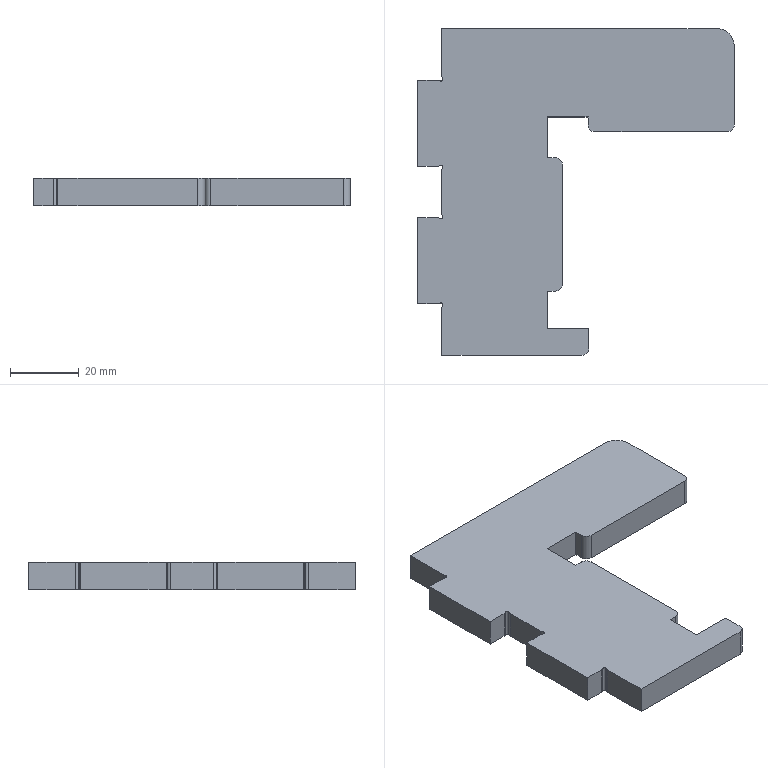Part | SolidWorks | features Fillet 2, FlatPattern 1, ICE 1, SMBaseFlange 1, SheetMetal 1 | 1 solid | 46 faces | box 92 x 95 x 8 mm | volume 40763 mm3 | plane 24 | cylinder 22 | commonest cylinder face diameters 4 x13 1 x8 10 x1
STEP:
#1=CARTESIAN_POINT('',(-1503.95,-54.15,0.));
#2=VERTEX_POINT('',#1);
#3=CARTESIAN_POINT('',(-1504.668,-53.7,0.));
#4=VERTEX_POINT('',#3);
#5=CARTESIAN_POINT('',(-1504.45,-54.15,0.));
#6=DIRECTION('',(0.,0.,1.));
#7=DIRECTION('',(1.,0.,0.));
#8=AXIS2_PLACEMENT_3D('',#5,#6,#7);
#9=CIRCLE('',#8,0.5);
#10=EDGE_CURVE('',#2,#4,#9,.T.);
#11=ORIENTED_EDGE('',*,*,#10,.F.);
#12=CARTESIAN_POINT('',(-1503.95,-54.15,8.));
#13=VERTEX_POINT('',#12);
#14=CARTESIAN_POINT('',(-1503.95,-54.15,0.));
#15=DIRECTION('',(0.,0.,1.));
#16=VECTOR('',#15,1000.);
#17=LINE('',#14,#16);
#18=EDGE_CURVE('',#2,#13,#17,.T.);
#19=ORIENTED_EDGE('',*,*,#18,.T.);
#20=CARTESIAN_POINT('',(-1504.668,-53.7,8.));
#21=VERTEX_POINT('',#20);
#22=CARTESIAN_POINT('',(-1504.45,-54.15,8.));
#23=DIRECTION('',(0.,0.,1.));
#24=DIRECTION('',(1.,0.,0.));
#25=AXIS2_PLACEMENT_3D('',#22,#23,#24);
#26=CIRCLE('',#25,0.5);
#27=EDGE_CURVE('',#13,#21,#26,.T.);
#28=ORIENTED_EDGE('',*,*,#27,.T.);
#29=CARTESIAN_POINT('',(-1504.668,-53.7,0.));
#30=DIRECTION('',(0.,0.,-1.));
#31=VECTOR('',#30,1000.);
#32=LINE('',#29,#31);
#33=EDGE_CURVE('',#21,#4,#32,.T.);
#34=ORIENTED_EDGE('',*,*,#33,.T.);
#35=EDGE_LOOP('',(#11,#19,#28,#34));
#36=FACE_OUTER_BOUND('',#35,.T.);
#37=CARTESIAN_POINT('',(-1504.45,-54.15,0.));
#38=DIRECTION('',(0.,0.,1.));
#39=DIRECTION('',(1.,0.,0.));
#40=AXIS2_PLACEMENT_3D('',#37,#38,#39);
#41=CYLINDRICAL_SURFACE('',#40,0.5);
#42=ADVANCED_FACE('',(#36),#41,.F.);
#43=CARTESIAN_POINT('',(-1503.95,11.35,0.));
#44=VERTEX_POINT('',#43);
#45=CARTESIAN_POINT('',(-1504.,11.568,0.));
#46=VERTEX_POINT('',#45);
#47=CARTESIAN_POINT('',(-1504.45,11.35,0.));
#48=DIRECTION('',(0.,0.,1.));
#49=DIRECTION('',(1.,0.,0.));
#50=AXIS2_PLACEMENT_3D('',#47,#48,#49);
#51=CIRCLE('',#50,0.5);
#52=EDGE_CURVE('',#44,#46,#51,.T.);
#53=ORIENTED_EDGE('',*,*,#52,.F.);
#54=CARTESIAN_POINT('',(-1503.95,11.35,8.));
#55=VERTEX_POINT('',#54);
#56=CARTESIAN_POINT('',(-1503.95,11.35,0.));
#57=DIRECTION('',(0.,0.,1.));
#58=VECTOR('',#57,1000.);
#59=LINE('',#56,#58);
#60=EDGE_CURVE('',#44,#55,#59,.T.);
#61=ORIENTED_EDGE('',*,*,#60,.T.);
#62=CARTESIAN_POINT('',(-1504.,11.568,8.));
#63=VERTEX_POINT('',#62);
#64=CARTESIAN_POINT('',(-1504.45,11.35,8.));
#65=DIRECTION('',(0.,0.,1.));
#66=DIRECTION('',(1.,0.,0.));
#67=AXIS2_PLACEMENT_3D('',#64,#65,#66);
#68=CIRCLE('',#67,0.5);
#69=EDGE_CURVE('',#55,#63,#68,.T.);
#70=ORIENTED_EDGE('',*,*,#69,.T.);
#71=CARTESIAN_POINT('',(-1504.,11.568,0.));
#72=DIRECTION('',(0.,0.,-1.));
#73=VECTOR('',#72,1000.);
#74=LINE('',#71,#73);
#75=EDGE_CURVE('',#63,#46,#74,.T.);
#76=ORIENTED_EDGE('',*,*,#75,.T.);
#77=EDGE_LOOP('',(#53,#61,#70,#76));
#78=FACE_OUTER_BOUND('',#77,.T.);
#79=CARTESIAN_POINT('',(-1504.45,11.35,0.));
#80=DIRECTION('',(0.,0.,1.));
#81=DIRECTION('',(1.,0.,0.));
#82=AXIS2_PLACEMENT_3D('',#79,#80,#81);
#83=CYLINDRICAL_SURFACE('',#82,0.5);
#84=ADVANCED_FACE('',(#78),#83,.F.);
#85=CARTESIAN_POINT('',(-1503.95,-14.15,0.));
#86=VERTEX_POINT('',#85);
#87=CARTESIAN_POINT('',(-1504.668,-13.7,0.));
#88=VERTEX_POINT('',#87);
#89=CARTESIAN_POINT('',(-1504.45,-14.15,0.));
#90=DIRECTION('',(0.,0.,1.));
#91=DIRECTION('',(1.,0.,0.));
#92=AXIS2_PLACEMENT_3D('',#89,#90,#91);
#93=CIRCLE('',#92,0.5);
#94=EDGE_CURVE('',#86,#88,#93,.T.);
#95=ORIENTED_EDGE('',*,*,#94,.F.);
#96=CARTESIAN_POINT('',(-1503.95,-14.15,8.));
#97=VERTEX_POINT('',#96);
#98=CARTESIAN_POINT('',(-1503.95,-14.15,0.));
#99=DIRECTION('',(0.,0.,1.));
#100=VECTOR('',#99,1000.);
#101=LINE('',#98,#100);
#102=EDGE_CURVE('',#86,#97,#101,.T.);
#103=ORIENTED_EDGE('',*,*,#102,.T.);
#104=CARTESIAN_POINT('',(-1504.668,-13.7,8.));
#105=VERTEX_POINT('',#104);
#106=CARTESIAN_POINT('',(-1504.45,-14.15,8.));
#107=DIRECTION('',(0.,0.,1.));
#108=DIRECTION('',(1.,0.,0.));
#109=AXIS2_PLACEMENT_3D('',#106,#107,#108);
#110=CIRCLE('',#109,0.5);
#111=EDGE_CURVE('',#97,#105,#110,.T.);
#112=ORIENTED_EDGE('',*,*,#111,.T.);
#113=CARTESIAN_POINT('',(-1504.668,-13.7,0.));
#114=DIRECTION('',(0.,0.,-1.));
#115=VECTOR('',#114,1000.);
#116=LINE('',#113,#115);
#117=EDGE_CURVE('',#105,#88,#116,.T.);
#118=ORIENTED_EDGE('',*,*,#117,.T.);
#119=EDGE_LOOP('',(#95,#103,#112,#118));
#120=FACE_OUTER_BOUND('',#119,.T.);
#121=CARTESIAN_POINT('',(-1504.45,-14.15,0.));
#122=DIRECTION('',(0.,0.,1.));
#123=DIRECTION('',(1.,0.,0.));
#124=AXIS2_PLACEMENT_3D('',#121,#122,#123);
#125=CYLINDRICAL_SURFACE('',#124,0.5);
#126=ADVANCED_FACE('',(#120),#125,.F.);
#127=CARTESIAN_POINT('',(-1503.95,-28.648,0.));
#128=VERTEX_POINT('',#127);
#129=CARTESIAN_POINT('',(-1504.,-28.43,0.));
#130=VERTEX_POINT('',#129);
#131=CARTESIAN_POINT('',(-1504.45,-28.648,0.));
#132=DIRECTION('',(0.,0.,1.));
#133=DIRECTION('',(1.,0.,0.));
#134=AXIS2_PLACEMENT_3D('',#131,#132,#133);
#135=CIRCLE('',#134,0.5);
#136=EDGE_CURVE('',#128,#130,#135,.T.);
#137=ORIENTED_EDGE('',*,*,#136,.F.);
#138=CARTESIAN_POINT('',(-1503.95,-28.648,8.));
#139=VERTEX_POINT('',#138);
#140=CARTESIAN_POINT('',(-1503.95,-28.648,0.));
#141=DIRECTION('',(0.,0.,1.));
#142=VECTOR('',#141,1000.);
#143=LINE('',#140,#142);
#144=EDGE_CURVE('',#128,#139,#143,.T.);
#145=ORIENTED_EDGE('',*,*,#144,.T.);
#146=CARTESIAN_POINT('',(-1504.,-28.43,8.));
#147=VERTEX_POINT('',#146);
#148=CARTESIAN_POINT('',(-1504.45,-28.648,8.));
#149=DIRECTION('',(0.,0.,1.));
#150=DIRECTION('',(1.,0.,0.));
#151=AXIS2_PLACEMENT_3D('',#148,#149,#150);
#152=CIRCLE('',#151,0.5);
#153=EDGE_CURVE('',#139,#147,#152,.T.);
#154=ORIENTED_EDGE('',*,*,#153,.T.);
#155=CARTESIAN_POINT('',(-1504.,-28.43,0.));
#156=DIRECTION('',(0.,0.,-1.));
#157=VECTOR('',#156,1000.);
#158=LINE('',#155,#157);
#159=EDGE_CURVE('',#147,#130,#158,.T.);
#160=ORIENTED_EDGE('',*,*,#159,.T.);
#161=EDGE_LOOP('',(#137,#145,#154,#160));
#162=FACE_OUTER_BOUND('',#161,.T.);
#163=CARTESIAN_POINT('',(-1504.45,-28.648,0.));
#164=DIRECTION('',(0.,0.,1.));
#165=DIRECTION('',(1.,0.,0.));
#166=AXIS2_PLACEMENT_3D('',#163,#164,#165);
#167=CYLINDRICAL_SURFACE('',#166,0.5);
#168=ADVANCED_FACE('',(#162),#167,.F.);
#169=CARTESIAN_POINT('',(-1504.2,26.1,0.));
#170=VERTEX_POINT('',#169);
#171=CARTESIAN_POINT('',(-1504.2,12.44,0.));
#172=VERTEX_POINT('',#171);
#173=CARTESIAN_POINT('',(-1504.2,26.1,0.));
#174=DIRECTION('',(0.,-1.,0.));
#175=VECTOR('',#174,1000.);
#176=LINE('',#173,#175);
#177=EDGE_CURVE('',#170,#172,#176,.T.);
#178=ORIENTED_EDGE('',*,*,#177,.T.);
#179=CARTESIAN_POINT('',(-1504.2,12.44,8.));
#180=VERTEX_POINT('',#179);
#181=CARTESIAN_POINT('',(-1504.2,12.44,8.));
#182=DIRECTION('',(0.,0.,1.));
#183=VECTOR('',#182,1000.);
#184=LINE('',#181,#183);
#185=EDGE_CURVE('',#172,#180,#184,.T.);
#186=ORIENTED_EDGE('',*,*,#185,.T.);
#187=CARTESIAN_POINT('',(-1504.2,26.1,8.));
#188=VERTEX_POINT('',#187);
#189=CARTESIAN_POINT('',(-1504.2,26.1,8.));
#190=DIRECTION('',(0.,-1.,0.));
#191=VECTOR('',#190,1000.);
#192=LINE('',#189,#191);
#193=EDGE_CURVE('',#188,#180,#192,.T.);
#194=ORIENTED_EDGE('',*,*,#193,.F.);
#195=CARTESIAN_POINT('',(-1504.2,26.1,8.));
#196=DIRECTION('',(0.,0.,-1.));
#197=VECTOR('',#196,1000.);
#198=LINE('',#195,#197);
#199=EDGE_CURVE('',#188,#170,#198,.T.);
#200=ORIENTED_EDGE('',*,*,#199,.T.);
#201=EDGE_LOOP('',(#178,#186,#194,#200));
#202=FACE_OUTER_BOUND('',#201,.T.);
#203=CARTESIAN_POINT('',(-1504.2,26.1,8.));
#204=DIRECTION('',(1.,0.,0.));
#205=DIRECTION('',(0.,0.,-1.));
#206=AXIS2_PLACEMENT_3D('',#203,#204,#205);
#207=PLANE('',#206);
#208=ADVANCED_FACE('',(#202),#207,.F.);
#209=CARTESIAN_POINT('',(-1505.54,11.1,8.));
#210=VERTEX_POINT('',#209);
#211=CARTESIAN_POINT('',(-1511.2,11.1,8.));
#212=VERTEX_POINT('',#211);
#213=CARTESIAN_POINT('',(-1511.2,11.1,8.));
#214=DIRECTION('',(-1.,0.,0.));
#215=VECTOR('',#214,1000.);
#216=LINE('',#213,#215);
#217=EDGE_CURVE('',#210,#212,#216,.T.);
#218=ORIENTED_EDGE('',*,*,#217,.F.);
#219=CARTESIAN_POINT('',(-1505.54,11.1,0.));
#220=VERTEX_POINT('',#219);
#221=CARTESIAN_POINT('',(-1505.54,11.1,0.));
#222=DIRECTION('',(0.,0.,-1.));
#223=VECTOR('',#222,1000.);
#224=LINE('',#221,#223);
#225=EDGE_CURVE('',#210,#220,#224,.T.);
#226=ORIENTED_EDGE('',*,*,#225,.T.);
#227=CARTESIAN_POINT('',(-1511.2,11.1,0.));
#228=VERTEX_POINT('',#227);
#229=CARTESIAN_POINT('',(-1511.2,11.1,0.));
#230=DIRECTION('',(-1.,0.,0.));
#231=VECTOR('',#230,1000.);
#232=LINE('',#229,#231);
#233=EDGE_CURVE('',#220,#228,#232,.T.);
#234=ORIENTED_EDGE('',*,*,#233,.T.);
#235=CARTESIAN_POINT('',(-1511.2,11.1,8.));
#236=DIRECTION('',(0.,0.,-1.));
#237=VECTOR('',#236,1000.);
#238=LINE('',#235,#237);
#239=EDGE_CURVE('',#212,#228,#238,.T.);
#240=ORIENTED_EDGE('',*,*,#239,.F.);
#241=EDGE_LOOP('',(#218,#226,#234,#240));
#242=FACE_OUTER_BOUND('',#241,.T.);
#243=CARTESIAN_POINT('',(-1511.2,11.1,8.));
#244=DIRECTION('',(0.,-1.,0.));
#245=DIRECTION('',(0.,0.,-1.));
#246=AXIS2_PLACEMENT_3D('',#243,#244,#245);
#247=PLANE('',#246);
#248=ADVANCED_FACE('',(#242),#247,.F.);
#249=CARTESIAN_POINT('',(-1511.2,-13.9,0.));
#250=VERTEX_POINT('',#249);
#251=CARTESIAN_POINT('',(-1505.54,-13.9,0.));
#252=VERTEX_POINT('',#251);
#253=CARTESIAN_POINT('',(-1504.2,-13.9,0.));
#254=DIRECTION('',(1.,0.,0.));
#255=VECTOR('',#254,1000.);
#256=LINE('',#253,#255);
#257=EDGE_CURVE('',#250,#252,#256,.T.);
#258=ORIENTED_EDGE('',*,*,#257,.T.);
#259=CARTESIAN_POINT('',(-1505.54,-13.9,8.));
#260=VERTEX_POINT('',#259);
#261=CARTESIAN_POINT('',(-1505.54,-13.9,8.));
#262=DIRECTION('',(0.,0.,1.));
#263=VECTOR('',#262,1000.);
#264=LINE('',#261,#263);
#265=EDGE_CURVE('',#252,#260,#264,.T.);
#266=ORIENTED_EDGE('',*,*,#265,.T.);
#267=CARTESIAN_POINT('',(-1511.2,-13.9,8.));
#268=VERTEX_POINT('',#267);
#269=CARTESIAN_POINT('',(-1504.2,-13.9,8.));
#270=DIRECTION('',(1.,0.,0.));
#271=VECTOR('',#270,1000.);
#272=LINE('',#269,#271);
#273=EDGE_CURVE('',#268,#260,#272,.T.);
#274=ORIENTED_EDGE('',*,*,#273,.F.);
#275=CARTESIAN_POINT('',(-1511.2,-13.9,8.));
#276=DIRECTION('',(0.,0.,-1.));
#277=VECTOR('',#276,1000.);
#278=LINE('',#275,#277);
#279=EDGE_CURVE('',#268,#250,#278,.T.);
#280=ORIENTED_EDGE('',*,*,#279,.T.);
#281=EDGE_LOOP('',(#258,#266,#274,#280));
#282=FACE_OUTER_BOUND('',#281,.T.);
#283=CARTESIAN_POINT('',(-1504.2,-13.9,8.));
#284=DIRECTION('',(0.,1.,0.));
#285=DIRECTION('',(0.,0.,1.));
#286=AXIS2_PLACEMENT_3D('',#283,#284,#285);
#287=PLANE('',#286);
#288=ADVANCED_FACE('',(#282),#287,.F.);
#289=CARTESIAN_POINT('',(-1504.2,-15.24,8.));
#290=VERTEX_POINT('',#289);
#291=CARTESIAN_POINT('',(-1504.2,-27.558,8.));
#292=VERTEX_POINT('',#291);
#293=CARTESIAN_POINT('',(-1504.2,-13.9,8.));
#294=DIRECTION('',(0.,-1.,0.));
#295=VECTOR('',#294,1000.);
#296=LINE('',#293,#295);
#297=EDGE_CURVE('',#290,#292,#296,.T.);
#298=ORIENTED_EDGE('',*,*,#297,.F.);
#299=CARTESIAN_POINT('',(-1504.2,-15.24,0.));
#300=VERTEX_POINT('',#299);
#301=CARTESIAN_POINT('',(-1504.2,-15.24,0.));
#302=DIRECTION('',(0.,0.,-1.));
#303=VECTOR('',#302,1000.);
#304=LINE('',#301,#303);
#305=EDGE_CURVE('',#290,#300,#304,.T.);
#306=ORIENTED_EDGE('',*,*,#305,.T.);
#307=CARTESIAN_POINT('',(-1504.2,-27.558,0.));
#308=VERTEX_POINT('',#307);
#309=CARTESIAN_POINT('',(-1504.2,-13.9,0.));
#310=DIRECTION('',(0.,-1.,0.));
#311=VECTOR('',#310,1000.);
#312=LINE('',#309,#311);
#313=EDGE_CURVE('',#300,#308,#312,.T.);
#314=ORIENTED_EDGE('',*,*,#313,.T.);
#315=CARTESIAN_POINT('',(-1504.2,-27.558,8.));
#316=DIRECTION('',(0.,0.,1.));
#317=VECTOR('',#316,1000.);
#318=LINE('',#315,#317);
#319=EDGE_CURVE('',#308,#292,#318,.T.);
#320=ORIENTED_EDGE('',*,*,#319,.T.);
#321=EDGE_LOOP('',(#298,#306,#314,#320));
#322=FACE_OUTER_BOUND('',#321,.T.);
#323=CARTESIAN_POINT('',(-1504.2,-13.9,8.));
#324=DIRECTION('',(1.,0.,0.));
#325=DIRECTION('',(0.,0.,-1.));
#326=AXIS2_PLACEMENT_3D('',#323,#324,#325);
#327=PLANE('',#326);
#328=ADVANCED_FACE('',(#322),#327,.F.);
#329=CARTESIAN_POINT('',(-1505.535,-28.9,8.));
#330=VERTEX_POINT('',#329);
#331=CARTESIAN_POINT('',(-1511.2,-28.9,8.));
#332=VERTEX_POINT('',#331);
#333=CARTESIAN_POINT('',(-1511.2,-28.9,8.));
#334=DIRECTION('',(-1.,0.,0.));
#335=VECTOR('',#334,1000.);
#336=LINE('',#333,#335);
#337=EDGE_CURVE('',#330,#332,#336,.T.);
#338=ORIENTED_EDGE('',*,*,#337,.F.);
#339=CARTESIAN_POINT('',(-1505.535,-28.9,0.));
#340=VERTEX_POINT('',#339);
#341=CARTESIAN_POINT('',(-1505.535,-28.9,0.));
#342=DIRECTION('',(0.,0.,-1.));
#343=VECTOR('',#342,1000.);
#344=LINE('',#341,#343);
#345=EDGE_CURVE('',#330,#340,#344,.T.);
#346=ORIENTED_EDGE('',*,*,#345,.T.);
#347=CARTESIAN_POINT('',(-1511.2,-28.9,0.));
#348=VERTEX_POINT('',#347);
#349=CARTESIAN_POINT('',(-1511.2,-28.9,0.));
#350=DIRECTION('',(-1.,0.,0.));
#351=VECTOR('',#350,1000.);
#352=LINE('',#349,#351);
#353=EDGE_CURVE('',#340,#348,#352,.T.);
#354=ORIENTED_EDGE('',*,*,#353,.T.);
#355=CARTESIAN_POINT('',(-1511.2,-28.9,8.));
#356=DIRECTION('',(0.,0.,-1.));
#357=VECTOR('',#356,1000.);
#358=LINE('',#355,#357);
#359=EDGE_CURVE('',#332,#348,#358,.T.);
#360=ORIENTED_EDGE('',*,*,#359,.F.);
#361=EDGE_LOOP('',(#338,#346,#354,#360));
#362=FACE_OUTER_BOUND('',#361,.T.);
#363=CARTESIAN_POINT('',(-1511.2,-28.9,8.));
#364=DIRECTION('',(0.,-1.,0.));
#365=DIRECTION('',(1.,0.,0.));
#366=AXIS2_PLACEMENT_3D('',#363,#364,#365);
#367=PLANE('',#366);
#368=ADVANCED_FACE('',(#362),#367,.F.);
#369=CARTESIAN_POINT('',(-1511.2,-53.9,0.));
#370=VERTEX_POINT('',#369);
#371=CARTESIAN_POINT('',(-1505.54,-53.9,0.));
#372=VERTEX_POINT('',#371);
#373=CARTESIAN_POINT('',(-1504.2,-53.9,0.));
#374=DIRECTION('',(1.,0.,0.));
#375=VECTOR('',#374,1000.);
#376=LINE('',#373,#375);
#377=EDGE_CURVE('',#370,#372,#376,.T.);
#378=ORIENTED_EDGE('',*,*,#377,.T.);
#379=CARTESIAN_POINT('',(-1505.54,-53.9,8.));
#380=VERTEX_POINT('',#379);
#381=CARTESIAN_POINT('',(-1505.54,-53.9,8.));
#382=DIRECTION('',(0.,0.,1.));
#383=VECTOR('',#382,1000.);
#384=LINE('',#381,#383);
#385=EDGE_CURVE('',#372,#380,#384,.T.);
#386=ORIENTED_EDGE('',*,*,#385,.T.);
#387=CARTESIAN_POINT('',(-1511.2,-53.9,8.));
#388=VERTEX_POINT('',#387);
#389=CARTESIAN_POINT('',(-1504.2,-53.9,8.));
#390=DIRECTION('',(1.,0.,0.));
#391=VECTOR('',#390,1000.);
#392=LINE('',#389,#391);
#393=EDGE_CURVE('',#388,#380,#392,.T.);
#394=ORIENTED_EDGE('',*,*,#393,.F.);
#395=CARTESIAN_POINT('',(-1511.2,-53.9,8.));
#396=DIRECTION('',(0.,0.,-1.));
#397=VECTOR('',#396,1000.);
#398=LINE('',#395,#397);
#399=EDGE_CURVE('',#388,#370,#398,.T.);
#400=ORIENTED_EDGE('',*,*,#399,.T.);
#401=EDGE_LOOP('',(#378,#386,#394,#400));
#402=FACE_OUTER_BOUND('',#401,.T.);
#403=CARTESIAN_POINT('',(-1504.2,-53.9,8.));
#404=DIRECTION('',(0.,1.,0.));
#405=DIRECTION('',(-1.,0.,0.));
#406=AXIS2_PLACEMENT_3D('',#403,#404,#405);
#407=PLANE('',#406);
#408=ADVANCED_FACE('',(#402),#407,.F.);
#409=CARTESIAN_POINT('',(-1504.2,-55.24,8.));
#410=VERTEX_POINT('',#409);
#411=CARTESIAN_POINT('',(-1504.2,-68.9,8.));
#412=VERTEX_POINT('',#411);
#413=CARTESIAN_POINT('',(-1504.2,-53.9,8.));
#414=DIRECTION('',(0.,-1.,0.));
#415=VECTOR('',#414,1000.);
#416=LINE('',#413,#415);
#417=EDGE_CURVE('',#410,#412,#416,.T.);
#418=ORIENTED_EDGE('',*,*,#417,.F.);
#419=CARTESIAN_POINT('',(-1504.2,-55.24,0.));
#420=VERTEX_POINT('',#419);
#421=CARTESIAN_POINT('',(-1504.2,-55.24,0.));
#422=DIRECTION('',(0.,0.,-1.));
#423=VECTOR('',#422,1000.);
#424=LINE('',#421,#423);
#425=EDGE_CURVE('',#410,#420,#424,.T.);
#426=ORIENTED_EDGE('',*,*,#425,.T.);
#427=CARTESIAN_POINT('',(-1504.2,-68.9,0.));
#428=VERTEX_POINT('',#427);
#429=CARTESIAN_POINT('',(-1504.2,-53.9,0.));
#430=DIRECTION('',(0.,-1.,0.));
#431=VECTOR('',#430,1000.);
#432=LINE('',#429,#431);
#433=EDGE_CURVE('',#420,#428,#432,.T.);
#434=ORIENTED_EDGE('',*,*,#433,.T.);
#435=CARTESIAN_POINT('',(-1504.2,-68.9,8.));
#436=DIRECTION('',(0.,0.,-1.));
#437=VECTOR('',#436,1000.);
#438=LINE('',#435,#437);
#439=EDGE_CURVE('',#412,#428,#438,.T.);
#440=ORIENTED_EDGE('',*,*,#439,.F.);
#441=EDGE_LOOP('',(#418,#426,#434,#440));
#442=FACE_OUTER_BOUND('',#441,.T.);
#443=CARTESIAN_POINT('',(-1504.2,-53.9,8.));
#444=DIRECTION('',(1.,0.,0.));
#445=DIRECTION('',(0.,0.,-1.));
#446=AXIS2_PLACEMENT_3D('',#443,#444,#445);
#447=PLANE('',#446);
#448=ADVANCED_FACE('',(#442),#447,.F.);
#449=CARTESIAN_POINT('',(-1419.2,-1.9,8.));
#450=VERTEX_POINT('',#449);
#451=CARTESIAN_POINT('',(-1419.2,21.1,8.));
#452=VERTEX_POINT('',#451);
#453=CARTESIAN_POINT('',(-1419.2,-3.9,8.));
#454=DIRECTION('',(0.,1.,0.));
#455=VECTOR('',#454,1000.);
#456=LINE('',#453,#455);
#457=EDGE_CURVE('',#450,#452,#456,.T.);
#458=ORIENTED_EDGE('',*,*,#457,.T.);
#459=CARTESIAN_POINT('',(-1424.2,26.1,8.));
#460=VERTEX_POINT('',#459);
#461=CARTESIAN_POINT('',(-1424.2,21.1,8.));
#462=DIRECTION('',(0.,0.,1.));
#463=DIRECTION('',(1.,0.,0.));
#464=AXIS2_PLACEMENT_3D('',#461,#462,#463);
#465=CIRCLE('',#464,5.);
#466=EDGE_CURVE('',#452,#460,#465,.T.);
#467=ORIENTED_EDGE('',*,*,#466,.T.);
#468=CARTESIAN_POINT('',(-1419.2,26.1,8.));
#469=DIRECTION('',(-1.,0.,0.));
#470=VECTOR('',#469,1000.);
#471=LINE('',#468,#470);
#472=EDGE_CURVE('',#460,#188,#471,.T.);
#473=ORIENTED_EDGE('',*,*,#472,.T.);
#474=ORIENTED_EDGE('',*,*,#193,.T.);
#475=CARTESIAN_POINT('',(-1502.2,12.44,8.));
#476=DIRECTION('',(0.,0.,1.));
#477=DIRECTION('',(1.,0.,0.));
#478=AXIS2_PLACEMENT_3D('',#475,#476,#477);
#479=CIRCLE('',#478,2.);
#480=EDGE_CURVE('',#180,#63,#479,.T.);
#481=ORIENTED_EDGE('',*,*,#480,.T.);
#482=ORIENTED_EDGE('',*,*,#69,.F.);
#483=CARTESIAN_POINT('',(-1504.668,10.9,8.));
#484=VERTEX_POINT('',#483);
#485=CARTESIAN_POINT('',(-1504.45,11.35,8.));
#486=DIRECTION('',(0.,0.,1.));
#487=DIRECTION('',(1.,0.,0.));
#488=AXIS2_PLACEMENT_3D('',#485,#486,#487);
#489=CIRCLE('',#488,0.5);
#490=EDGE_CURVE('',#484,#55,#489,.T.);
#491=ORIENTED_EDGE('',*,*,#490,.F.);
#492=CARTESIAN_POINT('',(-1505.54,9.1,8.));
#493=DIRECTION('',(0.,0.,1.));
#494=DIRECTION('',(1.,0.,0.));
#495=AXIS2_PLACEMENT_3D('',#492,#493,#494);
#496=CIRCLE('',#495,2.);
#497=EDGE_CURVE('',#484,#210,#496,.T.);
#498=ORIENTED_EDGE('',*,*,#497,.T.);
#499=ORIENTED_EDGE('',*,*,#217,.T.);
#500=CARTESIAN_POINT('',(-1511.2,-13.9,8.));
#501=DIRECTION('',(0.,-1.,0.));
#502=VECTOR('',#501,1000.);
#503=LINE('',#500,#502);
#504=EDGE_CURVE('',#212,#268,#503,.T.);
#505=ORIENTED_EDGE('',*,*,#504,.T.);
#506=ORIENTED_EDGE('',*,*,#273,.T.);
#507=CARTESIAN_POINT('',(-1505.54,-11.9,8.));
#508=DIRECTION('',(0.,0.,1.));
#509=DIRECTION('',(1.,0.,0.));
#510=AXIS2_PLACEMENT_3D('',#507,#508,#509);
#511=CIRCLE('',#510,2.);
#512=EDGE_CURVE('',#260,#105,#511,.T.);
#513=ORIENTED_EDGE('',*,*,#512,.T.);
#514=ORIENTED_EDGE('',*,*,#111,.F.);
#515=CARTESIAN_POINT('',(-1504.,-14.368,8.));
#516=VERTEX_POINT('',#515);
#517=CARTESIAN_POINT('',(-1504.45,-14.15,8.));
#518=DIRECTION('',(0.,0.,1.));
#519=DIRECTION('',(1.,0.,0.));
#520=AXIS2_PLACEMENT_3D('',#517,#518,#519);
#521=CIRCLE('',#520,0.5);
#522=EDGE_CURVE('',#516,#97,#521,.T.);
#523=ORIENTED_EDGE('',*,*,#522,.F.);
#524=CARTESIAN_POINT('',(-1502.2,-15.24,8.));
#525=DIRECTION('',(0.,0.,1.));
#526=DIRECTION('',(1.,0.,0.));
#527=AXIS2_PLACEMENT_3D('',#524,#525,#526);
#528=CIRCLE('',#527,2.);
#529=EDGE_CURVE('',#516,#290,#528,.T.);
#530=ORIENTED_EDGE('',*,*,#529,.T.);
#531=ORIENTED_EDGE('',*,*,#297,.T.);
#532=CARTESIAN_POINT('',(-1502.2,-27.558,8.));
#533=DIRECTION('',(0.,0.,1.));
#534=DIRECTION('',(1.,0.,0.));
#535=AXIS2_PLACEMENT_3D('',#532,#533,#534);
#536=CIRCLE('',#535,2.);
#537=EDGE_CURVE('',#292,#147,#536,.T.);
#538=ORIENTED_EDGE('',*,*,#537,.T.);
#539=ORIENTED_EDGE('',*,*,#153,.F.);
#540=CARTESIAN_POINT('',(-1504.667,-29.098,8.));
#541=VERTEX_POINT('',#540);
#542=CARTESIAN_POINT('',(-1504.45,-28.648,8.));
#543=DIRECTION('',(0.,0.,1.));
#544=DIRECTION('',(1.,0.,0.));
#545=AXIS2_PLACEMENT_3D('',#542,#543,#544);
#546=CIRCLE('',#545,0.5);
#547=EDGE_CURVE('',#541,#139,#546,.T.);
#548=ORIENTED_EDGE('',*,*,#547,.F.);
#549=CARTESIAN_POINT('',(-1505.535,-30.9,8.));
#550=DIRECTION('',(0.,0.,1.));
#551=DIRECTION('',(1.,0.,0.));
#552=AXIS2_PLACEMENT_3D('',#549,#550,#551);
#553=CIRCLE('',#552,2.);
#554=EDGE_CURVE('',#541,#330,#553,.T.);
#555=ORIENTED_EDGE('',*,*,#554,.T.);
#556=ORIENTED_EDGE('',*,*,#337,.T.);
#557=CARTESIAN_POINT('',(-1511.2,-53.9,8.));
#558=DIRECTION('',(0.,-1.,0.));
#559=VECTOR('',#558,1000.);
#560=LINE('',#557,#559);
#561=EDGE_CURVE('',#332,#388,#560,.T.);
#562=ORIENTED_EDGE('',*,*,#561,.T.);
#563=ORIENTED_EDGE('',*,*,#393,.T.);
#564=CARTESIAN_POINT('',(-1505.54,-51.9,8.));
#565=DIRECTION('',(0.,0.,1.));
#566=DIRECTION('',(1.,0.,0.));
#567=AXIS2_PLACEMENT_3D('',#564,#565,#566);
#568=CIRCLE('',#567,2.);
#569=EDGE_CURVE('',#380,#21,#568,.T.);
#570=ORIENTED_EDGE('',*,*,#569,.T.);
#571=ORIENTED_EDGE('',*,*,#27,.F.);
#572=CARTESIAN_POINT('',(-1504.,-54.368,8.));
#573=VERTEX_POINT('',#572);
#574=CARTESIAN_POINT('',(-1504.45,-54.15,8.));
#575=DIRECTION('',(0.,0.,1.));
#576=DIRECTION('',(1.,0.,0.));
#577=AXIS2_PLACEMENT_3D('',#574,#575,#576);
#578=CIRCLE('',#577,0.5);
#579=EDGE_CURVE('',#573,#13,#578,.T.);
#580=ORIENTED_EDGE('',*,*,#579,.F.);
#581=CARTESIAN_POINT('',(-1502.2,-55.24,8.));
#582=DIRECTION('',(0.,0.,1.));
#583=DIRECTION('',(1.,0.,0.));
#584=AXIS2_PLACEMENT_3D('',#581,#582,#583);
#585=CIRCLE('',#584,2.);
#586=EDGE_CURVE('',#573,#410,#585,.T.);
#587=ORIENTED_EDGE('',*,*,#586,.T.);
#588=ORIENTED_EDGE('',*,*,#417,.T.);
#589=CARTESIAN_POINT('',(-1463.5,-68.9,8.));
#590=VERTEX_POINT('',#589);
#591=CARTESIAN_POINT('',(-1461.5,-68.9,8.));
#592=DIRECTION('',(1.,0.,0.));
#593=VECTOR('',#592,1000.);
#594=LINE('',#591,#593);
#595=EDGE_CURVE('',#412,#590,#594,.T.);
#596=ORIENTED_EDGE('',*,*,#595,.T.);
#597=CARTESIAN_POINT('',(-1461.5,-66.9,8.));
#598=VERTEX_POINT('',#597);
#599=CARTESIAN_POINT('',(-1463.5,-66.9,8.));
#600=DIRECTION('',(0.,0.,1.));
#601=DIRECTION('',(1.,0.,0.));
#602=AXIS2_PLACEMENT_3D('',#599,#600,#601);
#603=CIRCLE('',#602,2.);
#604=EDGE_CURVE('',#590,#598,#603,.T.);
#605=ORIENTED_EDGE('',*,*,#604,.T.);
#606=CARTESIAN_POINT('',(-1461.5,-61.,8.));
#607=VERTEX_POINT('',#606);
#608=CARTESIAN_POINT('',(-1461.5,-61.,8.));
#609=DIRECTION('',(0.,1.,0.));
#610=VECTOR('',#609,1000.);
#611=LINE('',#608,#610);
#612=EDGE_CURVE('',#598,#607,#611,.T.);
#613=ORIENTED_EDGE('',*,*,#612,.T.);
#614=CARTESIAN_POINT('',(-1473.5,-61.,8.));
#615=VERTEX_POINT('',#614);
#616=CARTESIAN_POINT('',(-1461.5,-61.,8.));
#617=DIRECTION('',(-1.,0.,0.));
#618=VECTOR('',#617,1000.);
#619=LINE('',#616,#618);
#620=EDGE_CURVE('',#607,#615,#619,.T.);
#621=ORIENTED_EDGE('',*,*,#620,.T.);
#622=CARTESIAN_POINT('',(-1473.5,-50.2,8.));
#623=VERTEX_POINT('',#622);
#624=CARTESIAN_POINT('',(-1473.5,-61.,8.));
#625=DIRECTION('',(0.,1.,0.));
#626=VECTOR('',#625,1000.);
#627=LINE('',#624,#626);
#628=EDGE_CURVE('',#615,#623,#627,.T.);
#629=ORIENTED_EDGE('',*,*,#628,.T.);
#630=CARTESIAN_POINT('',(-1471.2,-50.2,8.));
#631=VERTEX_POINT('',#630);
#632=CARTESIAN_POINT('',(-1473.5,-50.2,8.));
#633=DIRECTION('',(1.,0.,0.));
#634=VECTOR('',#633,1000.);
#635=LINE('',#632,#634);
#636=EDGE_CURVE('',#623,#631,#635,.T.);
#637=ORIENTED_EDGE('',*,*,#636,.T.);
#638=CARTESIAN_POINT('',(-1469.2,-48.2,8.));
#639=VERTEX_POINT('',#638);
#640=CARTESIAN_POINT('',(-1471.2,-48.2,8.));
#641=DIRECTION('',(0.,0.,1.));
#642=DIRECTION('',(1.,0.,0.));
#643=AXIS2_PLACEMENT_3D('',#640,#641,#642);
#644=CIRCLE('',#643,2.);
#645=EDGE_CURVE('',#631,#639,#644,.T.);
#646=ORIENTED_EDGE('',*,*,#645,.T.);
#647=CARTESIAN_POINT('',(-1469.2,-13.4,8.));
#648=VERTEX_POINT('',#647);
#649=CARTESIAN_POINT('',(-1469.2,-50.2,8.));
#650=DIRECTION('',(0.,1.,0.));
#651=VECTOR('',#650,1000.);
#652=LINE('',#649,#651);
#653=EDGE_CURVE('',#639,#648,#652,.T.);
#654=ORIENTED_EDGE('',*,*,#653,.T.);
#655=CARTESIAN_POINT('',(-1471.2,-11.4,8.));
#656=VERTEX_POINT('',#655);
#657=CARTESIAN_POINT('',(-1471.2,-13.4,8.));
#658=DIRECTION('',(0.,0.,1.));
#659=DIRECTION('',(1.,0.,0.));
#660=AXIS2_PLACEMENT_3D('',#657,#658,#659);
#661=CIRCLE('',#660,2.);
#662=EDGE_CURVE('',#648,#656,#661,.T.);
#663=ORIENTED_EDGE('',*,*,#662,.T.);
#664=CARTESIAN_POINT('',(-1473.5,-11.4,8.));
#665=VERTEX_POINT('',#664);
#666=CARTESIAN_POINT('',(-1469.2,-11.4,8.));
#667=DIRECTION('',(-1.,0.,0.));
#668=VECTOR('',#667,1000.);
#669=LINE('',#666,#668);
#670=EDGE_CURVE('',#656,#665,#669,.T.);
#671=ORIENTED_EDGE('',*,*,#670,.T.);
#672=CARTESIAN_POINT('',(-1473.5,0.4,8.));
#673=VERTEX_POINT('',#672);
#674=CARTESIAN_POINT('',(-1473.5,0.4,8.));
#675=DIRECTION('',(0.,1.,0.));
#676=VECTOR('',#675,1000.);
#677=LINE('',#674,#676);
#678=EDGE_CURVE('',#665,#673,#677,.T.);
#679=ORIENTED_EDGE('',*,*,#678,.T.);
#680=CARTESIAN_POINT('',(-1461.7,0.4,8.));
#681=VERTEX_POINT('',#680);
#682=CARTESIAN_POINT('',(-1461.7,0.4,8.));
#683=DIRECTION('',(1.,0.,0.));
#684=VECTOR('',#683,1000.);
#685=LINE('',#682,#684);
#686=EDGE_CURVE('',#673,#681,#685,.T.);
#687=ORIENTED_EDGE('',*,*,#686,.T.);
#688=CARTESIAN_POINT('',(-1461.7,-1.9,8.));
#689=VERTEX_POINT('',#688);
#690=CARTESIAN_POINT('',(-1461.7,-3.9,8.));
#691=DIRECTION('',(0.,-1.,0.));
#692=VECTOR('',#691,1000.);
#693=LINE('',#690,#692);
#694=EDGE_CURVE('',#681,#689,#693,.T.);
#695=ORIENTED_EDGE('',*,*,#694,.T.);
#696=CARTESIAN_POINT('',(-1459.7,-3.9,8.));
#697=VERTEX_POINT('',#696);
#698=CARTESIAN_POINT('',(-1459.7,-1.9,8.));
#699=DIRECTION('',(0.,0.,1.));
#700=DIRECTION('',(1.,0.,0.));
#701=AXIS2_PLACEMENT_3D('',#698,#699,#700);
#702=CIRCLE('',#701,2.);
#703=EDGE_CURVE('',#689,#697,#702,.T.);
#704=ORIENTED_EDGE('',*,*,#703,.T.);
#705=CARTESIAN_POINT('',(-1421.2,-3.9,8.));
#706=VERTEX_POINT('',#705);
#707=CARTESIAN_POINT('',(-1419.2,-3.9,8.));
#708=DIRECTION('',(1.,0.,0.));
#709=VECTOR('',#708,1000.);
#710=LINE('',#707,#709);
#711=EDGE_CURVE('',#697,#706,#710,.T.);
#712=ORIENTED_EDGE('',*,*,#711,.T.);
#713=CARTESIAN_POINT('',(-1421.2,-1.9,8.));
#714=DIRECTION('',(0.,0.,1.));
#715=DIRECTION('',(1.,0.,0.));
#716=AXIS2_PLACEMENT_3D('',#713,#714,#715);
#717=CIRCLE('',#716,2.);
#718=EDGE_CURVE('',#706,#450,#717,.T.);
#719=ORIENTED_EDGE('',*,*,#718,.T.);
#720=EDGE_LOOP('',(#458,#467,#473,#474,#481,#482,#491,#498,#499,#505,#506,#513,#514,#523,#530,#531,#538,#539,#548,#555,#556,#562,#563,#570,#571,#580,#587,#588,#596,#605,#613,#621,#629,#637,#646,#654,#663,#671,#679,#687,#695,#704,#712,#719));
#721=FACE_OUTER_BOUND('',#720,.T.);
#722=CARTESIAN_POINT('',(0.,0.,8.));
#723=DIRECTION('',(0.,0.,1.));
#724=DIRECTION('',(1.,0.,0.));
#725=AXIS2_PLACEMENT_3D('',#722,#723,#724);
#726=PLANE('',#725);
#727=ADVANCED_FACE('',(#721),#726,.T.);
#728=CARTESIAN_POINT('',(-1424.2,26.1,0.));
#729=VERTEX_POINT('',#728);
#730=CARTESIAN_POINT('',(-1419.2,26.1,0.));
#731=DIRECTION('',(-1.,0.,0.));
#732=VECTOR('',#731,1000.);
#733=LINE('',#730,#732);
#734=EDGE_CURVE('',#729,#170,#733,.T.);
#735=ORIENTED_EDGE('',*,*,#734,.F.);
#736=CARTESIAN_POINT('',(-1419.2,21.1,0.));
#737=VERTEX_POINT('',#736);
#738=CARTESIAN_POINT('',(-1424.2,21.1,0.));
#739=DIRECTION('',(0.,0.,-1.));
#740=DIRECTION('',(1.,0.,0.));
#741=AXIS2_PLACEMENT_3D('',#738,#739,#740);
#742=CIRCLE('',#741,5.);
#743=EDGE_CURVE('',#729,#737,#742,.T.);
#744=ORIENTED_EDGE('',*,*,#743,.T.);
#745=CARTESIAN_POINT('',(-1419.2,-1.9,0.));
#746=VERTEX_POINT('',#745);
#747=CARTESIAN_POINT('',(-1419.2,-3.9,0.));
#748=DIRECTION('',(0.,1.,0.));
#749=VECTOR('',#748,1000.);
#750=LINE('',#747,#749);
#751=EDGE_CURVE('',#746,#737,#750,.T.);
#752=ORIENTED_EDGE('',*,*,#751,.F.);
#753=CARTESIAN_POINT('',(-1421.2,-3.9,0.));
#754=VERTEX_POINT('',#753);
#755=CARTESIAN_POINT('',(-1421.2,-1.9,0.));
#756=DIRECTION('',(0.,0.,-1.));
#757=DIRECTION('',(1.,0.,0.));
#758=AXIS2_PLACEMENT_3D('',#755,#756,#757);
#759=CIRCLE('',#758,2.);
#760=EDGE_CURVE('',#746,#754,#759,.T.);
#761=ORIENTED_EDGE('',*,*,#760,.T.);
#762=CARTESIAN_POINT('',(-1459.7,-3.9,0.));
#763=VERTEX_POINT('',#762);
#764=CARTESIAN_POINT('',(-1419.2,-3.9,0.));
#765=DIRECTION('',(1.,0.,0.));
#766=VECTOR('',#765,1000.);
#767=LINE('',#764,#766);
#768=EDGE_CURVE('',#763,#754,#767,.T.);
#769=ORIENTED_EDGE('',*,*,#768,.F.);
#770=CARTESIAN_POINT('',(-1461.7,-1.9,0.));
#771=VERTEX_POINT('',#770);
#772=CARTESIAN_POINT('',(-1459.7,-1.9,0.));
#773=DIRECTION('',(0.,0.,-1.));
#774=DIRECTION('',(1.,0.,0.));
#775=AXIS2_PLACEMENT_3D('',#772,#773,#774);
#776=CIRCLE('',#775,2.);
#777=EDGE_CURVE('',#763,#771,#776,.T.);
#778=ORIENTED_EDGE('',*,*,#777,.T.);
#779=CARTESIAN_POINT('',(-1461.7,0.4,0.));
#780=VERTEX_POINT('',#779);
#781=CARTESIAN_POINT('',(-1461.7,-3.9,0.));
#782=DIRECTION('',(0.,-1.,0.));
#783=VECTOR('',#782,1000.);
#784=LINE('',#781,#783);
#785=EDGE_CURVE('',#780,#771,#784,.T.);
#786=ORIENTED_EDGE('',*,*,#785,.F.);
#787=CARTESIAN_POINT('',(-1473.5,0.4,0.));
#788=VERTEX_POINT('',#787);
#789=CARTESIAN_POINT('',(-1461.7,0.4,0.));
#790=DIRECTION('',(1.,0.,0.));
#791=VECTOR('',#790,1000.);
#792=LINE('',#789,#791);
#793=EDGE_CURVE('',#788,#780,#792,.T.);
#794=ORIENTED_EDGE('',*,*,#793,.F.);
#795=CARTESIAN_POINT('',(-1473.5,-11.4,0.));
#796=VERTEX_POINT('',#795);
#797=CARTESIAN_POINT('',(-1473.5,0.4,0.));
#798=DIRECTION('',(0.,1.,0.));
#799=VECTOR('',#798,1000.);
#800=LINE('',#797,#799);
#801=EDGE_CURVE('',#796,#788,#800,.T.);
#802=ORIENTED_EDGE('',*,*,#801,.F.);
#803=CARTESIAN_POINT('',(-1471.2,-11.4,0.));
#804=VERTEX_POINT('',#803);
#805=CARTESIAN_POINT('',(-1469.2,-11.4,0.));
#806=DIRECTION('',(-1.,0.,0.));
#807=VECTOR('',#806,1000.);
#808=LINE('',#805,#807);
#809=EDGE_CURVE('',#804,#796,#808,.T.);
#810=ORIENTED_EDGE('',*,*,#809,.F.);
#811=CARTESIAN_POINT('',(-1469.2,-13.4,0.));
#812=VERTEX_POINT('',#811);
#813=CARTESIAN_POINT('',(-1471.2,-13.4,0.));
#814=DIRECTION('',(0.,0.,-1.));
#815=DIRECTION('',(1.,0.,0.));
#816=AXIS2_PLACEMENT_3D('',#813,#814,#815);
#817=CIRCLE('',#816,2.);
#818=EDGE_CURVE('',#804,#812,#817,.T.);
#819=ORIENTED_EDGE('',*,*,#818,.T.);
#820=CARTESIAN_POINT('',(-1469.2,-48.2,0.));
#821=VERTEX_POINT('',#820);
#822=CARTESIAN_POINT('',(-1469.2,-50.2,0.));
#823=DIRECTION('',(0.,1.,0.));
#824=VECTOR('',#823,1000.);
#825=LINE('',#822,#824);
#826=EDGE_CURVE('',#821,#812,#825,.T.);
#827=ORIENTED_EDGE('',*,*,#826,.F.);
#828=CARTESIAN_POINT('',(-1471.2,-50.2,0.));
#829=VERTEX_POINT('',#828);
#830=CARTESIAN_POINT('',(-1471.2,-48.2,0.));
#831=DIRECTION('',(0.,0.,-1.));
#832=DIRECTION('',(1.,0.,0.));
#833=AXIS2_PLACEMENT_3D('',#830,#831,#832);
#834=CIRCLE('',#833,2.);
#835=EDGE_CURVE('',#821,#829,#834,.T.);
#836=ORIENTED_EDGE('',*,*,#835,.T.);
#837=CARTESIAN_POINT('',(-1473.5,-50.2,0.));
#838=VERTEX_POINT('',#837);
#839=CARTESIAN_POINT('',(-1473.5,-50.2,0.));
#840=DIRECTION('',(1.,0.,0.));
#841=VECTOR('',#840,1000.);
#842=LINE('',#839,#841);
#843=EDGE_CURVE('',#838,#829,#842,.T.);
#844=ORIENTED_EDGE('',*,*,#843,.F.);
#845=CARTESIAN_POINT('',(-1473.5,-61.,0.));
#846=VERTEX_POINT('',#845);
#847=CARTESIAN_POINT('',(-1473.5,-61.,0.));
#848=DIRECTION('',(0.,1.,0.));
#849=VECTOR('',#848,1000.);
#850=LINE('',#847,#849);
#851=EDGE_CURVE('',#846,#838,#850,.T.);
#852=ORIENTED_EDGE('',*,*,#851,.F.);
#853=CARTESIAN_POINT('',(-1461.5,-61.,0.));
#854=VERTEX_POINT('',#853);
#855=CARTESIAN_POINT('',(-1461.5,-61.,0.));
#856=DIRECTION('',(-1.,0.,0.));
#857=VECTOR('',#856,1000.);
#858=LINE('',#855,#857);
#859=EDGE_CURVE('',#854,#846,#858,.T.);
#860=ORIENTED_EDGE('',*,*,#859,.F.);
#861=CARTESIAN_POINT('',(-1461.5,-66.9,0.));
#862=VERTEX_POINT('',#861);
#863=CARTESIAN_POINT('',(-1461.5,-61.,0.));
#864=DIRECTION('',(0.,1.,0.));
#865=VECTOR('',#864,1000.);
#866=LINE('',#863,#865);
#867=EDGE_CURVE('',#862,#854,#866,.T.);
#868=ORIENTED_EDGE('',*,*,#867,.F.);
#869=CARTESIAN_POINT('',(-1463.5,-68.9,0.));
#870=VERTEX_POINT('',#869);
#871=CARTESIAN_POINT('',(-1463.5,-66.9,0.));
#872=DIRECTION('',(0.,0.,-1.));
#873=DIRECTION('',(1.,0.,0.));
#874=AXIS2_PLACEMENT_3D('',#871,#872,#873);
#875=CIRCLE('',#874,2.);
#876=EDGE_CURVE('',#862,#870,#875,.T.);
#877=ORIENTED_EDGE('',*,*,#876,.T.);
#878=CARTESIAN_POINT('',(-1461.5,-68.9,0.));
#879=DIRECTION('',(1.,0.,0.));
#880=VECTOR('',#879,1000.);
#881=LINE('',#878,#880);
#882=EDGE_CURVE('',#428,#870,#881,.T.);
#883=ORIENTED_EDGE('',*,*,#882,.F.);
#884=ORIENTED_EDGE('',*,*,#433,.F.);
#885=CARTESIAN_POINT('',(-1504.,-54.368,0.));
#886=VERTEX_POINT('',#885);
#887=CARTESIAN_POINT('',(-1502.2,-55.24,0.));
#888=DIRECTION('',(0.,0.,-1.));
#889=DIRECTION('',(1.,0.,0.));
#890=AXIS2_PLACEMENT_3D('',#887,#888,#889);
#891=CIRCLE('',#890,2.);
#892=EDGE_CURVE('',#420,#886,#891,.T.);
#893=ORIENTED_EDGE('',*,*,#892,.T.);
#894=CARTESIAN_POINT('',(-1504.45,-54.15,0.));
#895=DIRECTION('',(0.,0.,1.));
#896=DIRECTION('',(1.,0.,0.));
#897=AXIS2_PLACEMENT_3D('',#894,#895,#896);
#898=CIRCLE('',#897,0.5);
#899=EDGE_CURVE('',#886,#2,#898,.T.);
#900=ORIENTED_EDGE('',*,*,#899,.T.);
#901=ORIENTED_EDGE('',*,*,#10,.T.);
#902=CARTESIAN_POINT('',(-1505.54,-51.9,0.));
#903=DIRECTION('',(0.,0.,-1.));
#904=DIRECTION('',(1.,0.,0.));
#905=AXIS2_PLACEMENT_3D('',#902,#903,#904);
#906=CIRCLE('',#905,2.);
#907=EDGE_CURVE('',#4,#372,#906,.T.);
#908=ORIENTED_EDGE('',*,*,#907,.T.);
#909=ORIENTED_EDGE('',*,*,#377,.F.);
#910=CARTESIAN_POINT('',(-1511.2,-53.9,0.));
#911=DIRECTION('',(0.,-1.,0.));
#912=VECTOR('',#911,1000.);
#913=LINE('',#910,#912);
#914=EDGE_CURVE('',#348,#370,#913,.T.);
#915=ORIENTED_EDGE('',*,*,#914,.F.);
#916=ORIENTED_EDGE('',*,*,#353,.F.);
#917=CARTESIAN_POINT('',(-1504.667,-29.098,0.));
#918=VERTEX_POINT('',#917);
#919=CARTESIAN_POINT('',(-1505.535,-30.9,0.));
#920=DIRECTION('',(0.,0.,-1.));
#921=DIRECTION('',(1.,0.,0.));
#922=AXIS2_PLACEMENT_3D('',#919,#920,#921);
#923=CIRCLE('',#922,2.);
#924=EDGE_CURVE('',#340,#918,#923,.T.);
#925=ORIENTED_EDGE('',*,*,#924,.T.);
#926=CARTESIAN_POINT('',(-1504.45,-28.648,0.));
#927=DIRECTION('',(0.,0.,1.));
#928=DIRECTION('',(1.,0.,0.));
#929=AXIS2_PLACEMENT_3D('',#926,#927,#928);
#930=CIRCLE('',#929,0.5);
#931=EDGE_CURVE('',#918,#128,#930,.T.);
#932=ORIENTED_EDGE('',*,*,#931,.T.);
#933=ORIENTED_EDGE('',*,*,#136,.T.);
#934=CARTESIAN_POINT('',(-1502.2,-27.558,0.));
#935=DIRECTION('',(0.,0.,-1.));
#936=DIRECTION('',(1.,0.,0.));
#937=AXIS2_PLACEMENT_3D('',#934,#935,#936);
#938=CIRCLE('',#937,2.);
#939=EDGE_CURVE('',#130,#308,#938,.T.);
#940=ORIENTED_EDGE('',*,*,#939,.T.);
#941=ORIENTED_EDGE('',*,*,#313,.F.);
#942=CARTESIAN_POINT('',(-1504.,-14.368,0.));
#943=VERTEX_POINT('',#942);
#944=CARTESIAN_POINT('',(-1502.2,-15.24,0.));
#945=DIRECTION('',(0.,0.,-1.));
#946=DIRECTION('',(1.,0.,0.));
#947=AXIS2_PLACEMENT_3D('',#944,#945,#946);
#948=CIRCLE('',#947,2.);
#949=EDGE_CURVE('',#300,#943,#948,.T.);
#950=ORIENTED_EDGE('',*,*,#949,.T.);
#951=CARTESIAN_POINT('',(-1504.45,-14.15,0.));
#952=DIRECTION('',(0.,0.,1.));
#953=DIRECTION('',(1.,0.,0.));
#954=AXIS2_PLACEMENT_3D('',#951,#952,#953);
#955=CIRCLE('',#954,0.5);
#956=EDGE_CURVE('',#943,#86,#955,.T.);
#957=ORIENTED_EDGE('',*,*,#956,.T.);
#958=ORIENTED_EDGE('',*,*,#94,.T.);
#959=CARTESIAN_POINT('',(-1505.54,-11.9,0.));
#960=DIRECTION('',(0.,0.,-1.));
#961=DIRECTION('',(1.,0.,0.));
#962=AXIS2_PLACEMENT_3D('',#959,#960,#961);
#963=CIRCLE('',#962,2.);
#964=EDGE_CURVE('',#88,#252,#963,.T.);
#965=ORIENTED_EDGE('',*,*,#964,.T.);
#966=ORIENTED_EDGE('',*,*,#257,.F.);
#967=CARTESIAN_POINT('',(-1511.2,-13.9,0.));
#968=DIRECTION('',(0.,-1.,0.));
#969=VECTOR('',#968,1000.);
#970=LINE('',#967,#969);
#971=EDGE_CURVE('',#228,#250,#970,.T.);
#972=ORIENTED_EDGE('',*,*,#971,.F.);
#973=ORIENTED_EDGE('',*,*,#233,.F.);
#974=CARTESIAN_POINT('',(-1504.668,10.9,0.));
#975=VERTEX_POINT('',#974);
#976=CARTESIAN_POINT('',(-1505.54,9.1,0.));
#977=DIRECTION('',(0.,0.,-1.));
#978=DIRECTION('',(1.,0.,0.));
#979=AXIS2_PLACEMENT_3D('',#976,#977,#978);
#980=CIRCLE('',#979,2.);
#981=EDGE_CURVE('',#220,#975,#980,.T.);
#982=ORIENTED_EDGE('',*,*,#981,.T.);
#983=CARTESIAN_POINT('',(-1504.45,11.35,0.));
#984=DIRECTION('',(0.,0.,1.));
#985=DIRECTION('',(1.,0.,0.));
#986=AXIS2_PLACEMENT_3D('',#983,#984,#985);
#987=CIRCLE('',#986,0.5);
#988=EDGE_CURVE('',#975,#44,#987,.T.);
#989=ORIENTED_EDGE('',*,*,#988,.T.);
#990=ORIENTED_EDGE('',*,*,#52,.T.);
#991=CARTESIAN_POINT('',(-1502.2,12.44,0.));
#992=DIRECTION('',(0.,0.,-1.));
#993=DIRECTION('',(1.,0.,0.));
#994=AXIS2_PLACEMENT_3D('',#991,#992,#993);
#995=CIRCLE('',#994,2.);
#996=EDGE_CURVE('',#46,#172,#995,.T.);
#997=ORIENTED_EDGE('',*,*,#996,.T.);
#998=ORIENTED_EDGE('',*,*,#177,.F.);
#999=EDGE_LOOP('',(#735,#744,#752,#761,#769,#778,#786,#794,#802,#810,#819,#827,#836,#844,#852,#860,#868,#877,#883,#884,#893,#900,#901,#908,#909,#915,#916,#925,#932,#933,#940,#941,#950,#957,#958,#965,#966,#972,#973,#982,#989,#990,#997,#998));
#1000=FACE_OUTER_BOUND('',#999,.T.);
#1001=CARTESIAN_POINT('',(0.,0.,0.));
#1002=DIRECTION('',(0.,0.,1.));
#1003=DIRECTION('',(1.,0.,0.));
#1004=AXIS2_PLACEMENT_3D('',#1001,#1002,#1003);
#1005=PLANE('',#1004);
#1006=ADVANCED_FACE('',(#1000),#1005,.F.);
#1007=ORIENTED_EDGE('',*,*,#826,.T.);
#1008=CARTESIAN_POINT('',(-1469.2,-13.4,8.));
#1009=DIRECTION('',(0.,0.,1.));
#1010=VECTOR('',#1009,1000.);
#1011=LINE('',#1008,#1010);
#1012=EDGE_CURVE('',#812,#648,#1011,.T.);
#1013=ORIENTED_EDGE('',*,*,#1012,.T.);
#1014=ORIENTED_EDGE('',*,*,#653,.F.);
#1015=CARTESIAN_POINT('',(-1469.2,-48.2,8.));
#1016=DIRECTION('',(0.,0.,-1.));
#1017=VECTOR('',#1016,1000.);
#1018=LINE('',#1015,#1017);
#1019=EDGE_CURVE('',#639,#821,#1018,.T.);
#1020=ORIENTED_EDGE('',*,*,#1019,.T.);
#1021=EDGE_LOOP('',(#1007,#1013,#1014,#1020));
#1022=FACE_OUTER_BOUND('',#1021,.T.);
#1023=CARTESIAN_POINT('',(-1469.2,-50.2,8.));
#1024=DIRECTION('',(-1.,0.,0.));
#1025=DIRECTION('',(0.,0.,1.));
#1026=AXIS2_PLACEMENT_3D('',#1023,#1024,#1025);
#1027=PLANE('',#1026);
#1028=ADVANCED_FACE('',(#1022),#1027,.F.);
#1029=ORIENTED_EDGE('',*,*,#670,.F.);
#1030=CARTESIAN_POINT('',(-1471.2,-11.4,8.));
#1031=DIRECTION('',(0.,0.,-1.));
#1032=VECTOR('',#1031,1000.);
#1033=LINE('',#1030,#1032);
#1034=EDGE_CURVE('',#656,#804,#1033,.T.);
#1035=ORIENTED_EDGE('',*,*,#1034,.T.);
#1036=ORIENTED_EDGE('',*,*,#809,.T.);
#1037=CARTESIAN_POINT('',(-1473.5,-11.4,8.));
#1038=DIRECTION('',(0.,0.,-1.));
#1039=VECTOR('',#1038,1000.);
#1040=LINE('',#1037,#1039);
#1041=EDGE_CURVE('',#665,#796,#1040,.T.);
#1042=ORIENTED_EDGE('',*,*,#1041,.F.);
#1043=EDGE_LOOP('',(#1029,#1035,#1036,#1042));
#1044=FACE_OUTER_BOUND('',#1043,.T.);
#1045=CARTESIAN_POINT('',(-1469.2,-11.4,8.));
#1046=DIRECTION('',(0.,-1.,0.));
#1047=DIRECTION('',(1.,0.,0.));
#1048=AXIS2_PLACEMENT_3D('',#1045,#1046,#1047);
#1049=PLANE('',#1048);
#1050=ADVANCED_FACE('',(#1044),#1049,.F.);
#1051=ORIENTED_EDGE('',*,*,#801,.T.);
#1052=CARTESIAN_POINT('',(-1473.5,0.4,8.));
#1053=DIRECTION('',(0.,0.,-1.));
#1054=VECTOR('',#1053,1000.);
#1055=LINE('',#1052,#1054);
#1056=EDGE_CURVE('',#673,#788,#1055,.T.);
#1057=ORIENTED_EDGE('',*,*,#1056,.F.);
#1058=ORIENTED_EDGE('',*,*,#678,.F.);
#1059=ORIENTED_EDGE('',*,*,#1041,.T.);
#1060=EDGE_LOOP('',(#1051,#1057,#1058,#1059));
#1061=FACE_OUTER_BOUND('',#1060,.T.);
#1062=CARTESIAN_POINT('',(-1473.5,0.4,8.));
#1063=DIRECTION('',(-1.,0.,0.));
#1064=DIRECTION('',(0.,0.,1.));
#1065=AXIS2_PLACEMENT_3D('',#1062,#1063,#1064);
#1066=PLANE('',#1065);
#1067=ADVANCED_FACE('',(#1061),#1066,.F.);
#1068=ORIENTED_EDGE('',*,*,#793,.T.);
#1069=CARTESIAN_POINT('',(-1461.7,0.4,8.));
#1070=DIRECTION('',(0.,0.,-1.));
#1071=VECTOR('',#1070,1000.);
#1072=LINE('',#1069,#1071);
#1073=EDGE_CURVE('',#681,#780,#1072,.T.);
#1074=ORIENTED_EDGE('',*,*,#1073,.F.);
#1075=ORIENTED_EDGE('',*,*,#686,.F.);
#1076=ORIENTED_EDGE('',*,*,#1056,.T.);
#1077=EDGE_LOOP('',(#1068,#1074,#1075,#1076));
#1078=FACE_OUTER_BOUND('',#1077,.T.);
#1079=CARTESIAN_POINT('',(-1461.7,0.4,8.));
#1080=DIRECTION('',(0.,1.,0.));
#1081=DIRECTION('',(-1.,0.,0.));
#1082=AXIS2_PLACEMENT_3D('',#1079,#1080,#1081);
#1083=PLANE('',#1082);
#1084=ADVANCED_FACE('',(#1078),#1083,.F.);
#1085=ORIENTED_EDGE('',*,*,#785,.T.);
#1086=CARTESIAN_POINT('',(-1461.7,-1.9,8.));
#1087=DIRECTION('',(0.,0.,1.));
#1088=VECTOR('',#1087,1000.);
#1089=LINE('',#1086,#1088);
#1090=EDGE_CURVE('',#771,#689,#1089,.T.);
#1091=ORIENTED_EDGE('',*,*,#1090,.T.);
#1092=ORIENTED_EDGE('',*,*,#694,.F.);
#1093=ORIENTED_EDGE('',*,*,#1073,.T.);
#1094=EDGE_LOOP('',(#1085,#1091,#1092,#1093));
#1095=FACE_OUTER_BOUND('',#1094,.T.);
#1096=CARTESIAN_POINT('',(-1461.7,-3.9,8.));
#1097=DIRECTION('',(1.,0.,0.));
#1098=DIRECTION('',(0.,0.,-1.));
#1099=AXIS2_PLACEMENT_3D('',#1096,#1097,#1098);
#1100=PLANE('',#1099);
#1101=ADVANCED_FACE('',(#1095),#1100,.F.);
#1102=ORIENTED_EDGE('',*,*,#768,.T.);
#1103=CARTESIAN_POINT('',(-1421.2,-3.9,8.));
#1104=DIRECTION('',(0.,0.,1.));
#1105=VECTOR('',#1104,1000.);
#1106=LINE('',#1103,#1105);
#1107=EDGE_CURVE('',#754,#706,#1106,.T.);
#1108=ORIENTED_EDGE('',*,*,#1107,.T.);
#1109=ORIENTED_EDGE('',*,*,#711,.F.);
#1110=CARTESIAN_POINT('',(-1459.7,-3.9,8.));
#1111=DIRECTION('',(0.,0.,-1.));
#1112=VECTOR('',#1111,1000.);
#1113=LINE('',#1110,#1112);
#1114=EDGE_CURVE('',#697,#763,#1113,.T.);
#1115=ORIENTED_EDGE('',*,*,#1114,.T.);
#1116=EDGE_LOOP('',(#1102,#1108,#1109,#1115));
#1117=FACE_OUTER_BOUND('',#1116,.T.);
#1118=CARTESIAN_POINT('',(-1419.2,-3.9,8.));
#1119=DIRECTION('',(0.,1.,0.));
#1120=DIRECTION('',(0.,0.,1.));
#1121=AXIS2_PLACEMENT_3D('',#1118,#1119,#1120);
#1122=PLANE('',#1121);
#1123=ADVANCED_FACE('',(#1117),#1122,.F.);
#1124=ORIENTED_EDGE('',*,*,#751,.T.);
#1125=CARTESIAN_POINT('',(-1419.2,21.1,8.));
#1126=DIRECTION('',(0.,0.,1.));
#1127=VECTOR('',#1126,1000.);
#1128=LINE('',#1125,#1127);
#1129=EDGE_CURVE('',#737,#452,#1128,.T.);
#1130=ORIENTED_EDGE('',*,*,#1129,.T.);
#1131=ORIENTED_EDGE('',*,*,#457,.F.);
#1132=CARTESIAN_POINT('',(-1419.2,-1.9,8.));
#1133=DIRECTION('',(0.,0.,-1.));
#1134=VECTOR('',#1133,1000.);
#1135=LINE('',#1132,#1134);
#1136=EDGE_CURVE('',#450,#746,#1135,.T.);
#1137=ORIENTED_EDGE('',*,*,#1136,.T.);
#1138=EDGE_LOOP('',(#1124,#1130,#1131,#1137));
#1139=FACE_OUTER_BOUND('',#1138,.T.);
#1140=CARTESIAN_POINT('',(-1419.2,-3.9,8.));
#1141=DIRECTION('',(-1.,0.,0.));
#1142=DIRECTION('',(0.,0.,1.));
#1143=AXIS2_PLACEMENT_3D('',#1140,#1141,#1142);
#1144=PLANE('',#1143);
#1145=ADVANCED_FACE('',(#1139),#1144,.F.);
#1146=ORIENTED_EDGE('',*,*,#472,.F.);
#1147=CARTESIAN_POINT('',(-1424.2,26.1,8.));
#1148=DIRECTION('',(0.,0.,-1.));
#1149=VECTOR('',#1148,1000.);
#1150=LINE('',#1147,#1149);
#1151=EDGE_CURVE('',#460,#729,#1150,.T.);
#1152=ORIENTED_EDGE('',*,*,#1151,.T.);
#1153=ORIENTED_EDGE('',*,*,#734,.T.);
#1154=ORIENTED_EDGE('',*,*,#199,.F.);
#1155=EDGE_LOOP('',(#1146,#1152,#1153,#1154));
#1156=FACE_OUTER_BOUND('',#1155,.T.);
#1157=CARTESIAN_POINT('',(-1419.2,26.1,8.));
#1158=DIRECTION('',(0.,-1.,0.));
#1159=DIRECTION('',(1.,0.,0.));
#1160=AXIS2_PLACEMENT_3D('',#1157,#1158,#1159);
#1161=PLANE('',#1160);
#1162=ADVANCED_FACE('',(#1156),#1161,.F.);
#1163=ORIENTED_EDGE('',*,*,#971,.T.);
#1164=ORIENTED_EDGE('',*,*,#279,.F.);
#1165=ORIENTED_EDGE('',*,*,#504,.F.);
#1166=ORIENTED_EDGE('',*,*,#239,.T.);
#1167=EDGE_LOOP('',(#1163,#1164,#1165,#1166));
#1168=FACE_OUTER_BOUND('',#1167,.T.);
#1169=CARTESIAN_POINT('',(-1511.2,-13.9,8.));
#1170=DIRECTION('',(1.,0.,0.));
#1171=DIRECTION('',(0.,0.,-1.));
#1172=AXIS2_PLACEMENT_3D('',#1169,#1170,#1171);
#1173=PLANE('',#1172);
#1174=ADVANCED_FACE('',(#1168),#1173,.F.);
#1175=ORIENTED_EDGE('',*,*,#914,.T.);
#1176=ORIENTED_EDGE('',*,*,#399,.F.);
#1177=ORIENTED_EDGE('',*,*,#561,.F.);
#1178=ORIENTED_EDGE('',*,*,#359,.T.);
#1179=EDGE_LOOP('',(#1175,#1176,#1177,#1178));
#1180=FACE_OUTER_BOUND('',#1179,.T.);
#1181=CARTESIAN_POINT('',(-1511.2,-53.9,8.));
#1182=DIRECTION('',(1.,0.,0.));
#1183=DIRECTION('',(0.,0.,-1.));
#1184=AXIS2_PLACEMENT_3D('',#1181,#1182,#1183);
#1185=PLANE('',#1184);
#1186=ADVANCED_FACE('',(#1180),#1185,.F.);
#1187=ORIENTED_EDGE('',*,*,#882,.T.);
#1188=CARTESIAN_POINT('',(-1463.5,-68.9,8.));
#1189=DIRECTION('',(0.,0.,1.));
#1190=VECTOR('',#1189,1000.);
#1191=LINE('',#1188,#1190);
#1192=EDGE_CURVE('',#870,#590,#1191,.T.);
#1193=ORIENTED_EDGE('',*,*,#1192,.T.);
#1194=ORIENTED_EDGE('',*,*,#595,.F.);
#1195=ORIENTED_EDGE('',*,*,#439,.T.);
#1196=EDGE_LOOP('',(#1187,#1193,#1194,#1195));
#1197=FACE_OUTER_BOUND('',#1196,.T.);
#1198=CARTESIAN_POINT('',(-1461.5,-68.9,8.));
#1199=DIRECTION('',(0.,1.,0.));
#1200=DIRECTION('',(0.,0.,1.));
#1201=AXIS2_PLACEMENT_3D('',#1198,#1199,#1200);
#1202=PLANE('',#1201);
#1203=ADVANCED_FACE('',(#1197),#1202,.F.);
#1204=ORIENTED_EDGE('',*,*,#612,.F.);
#1205=CARTESIAN_POINT('',(-1461.5,-66.9,8.));
#1206=DIRECTION('',(0.,0.,-1.));
#1207=VECTOR('',#1206,1000.);
#1208=LINE('',#1205,#1207);
#1209=EDGE_CURVE('',#598,#862,#1208,.T.);
#1210=ORIENTED_EDGE('',*,*,#1209,.T.);
#1211=ORIENTED_EDGE('',*,*,#867,.T.);
#1212=CARTESIAN_POINT('',(-1461.5,-61.,8.));
#1213=DIRECTION('',(0.,0.,-1.));
#1214=VECTOR('',#1213,1000.);
#1215=LINE('',#1212,#1214);
#1216=EDGE_CURVE('',#607,#854,#1215,.T.);
#1217=ORIENTED_EDGE('',*,*,#1216,.F.);
#1218=EDGE_LOOP('',(#1204,#1210,#1211,#1217));
#1219=FACE_OUTER_BOUND('',#1218,.T.);
#1220=CARTESIAN_POINT('',(-1461.5,-61.,8.));
#1221=DIRECTION('',(-1.,0.,0.));
#1222=DIRECTION('',(0.,0.,1.));
#1223=AXIS2_PLACEMENT_3D('',#1220,#1221,#1222);
#1224=PLANE('',#1223);
#1225=ADVANCED_FACE('',(#1219),#1224,.F.);
#1226=ORIENTED_EDGE('',*,*,#859,.T.);
#1227=CARTESIAN_POINT('',(-1473.5,-61.,8.));
#1228=DIRECTION('',(0.,0.,-1.));
#1229=VECTOR('',#1228,1000.);
#1230=LINE('',#1227,#1229);
#1231=EDGE_CURVE('',#615,#846,#1230,.T.);
#1232=ORIENTED_EDGE('',*,*,#1231,.F.);
#1233=ORIENTED_EDGE('',*,*,#620,.F.);
#1234=ORIENTED_EDGE('',*,*,#1216,.T.);
#1235=EDGE_LOOP('',(#1226,#1232,#1233,#1234));
#1236=FACE_OUTER_BOUND('',#1235,.T.);
#1237=CARTESIAN_POINT('',(-1461.5,-61.,8.));
#1238=DIRECTION('',(0.,-1.,0.));
#1239=DIRECTION('',(0.,0.,-1.));
#1240=AXIS2_PLACEMENT_3D('',#1237,#1238,#1239);
#1241=PLANE('',#1240);
#1242=ADVANCED_FACE('',(#1236),#1241,.F.);
#1243=ORIENTED_EDGE('',*,*,#851,.T.);
#1244=CARTESIAN_POINT('',(-1473.5,-50.2,8.));
#1245=DIRECTION('',(0.,0.,-1.));
#1246=VECTOR('',#1245,1000.);
#1247=LINE('',#1244,#1246);
#1248=EDGE_CURVE('',#623,#838,#1247,.T.);
#1249=ORIENTED_EDGE('',*,*,#1248,.F.);
#1250=ORIENTED_EDGE('',*,*,#628,.F.);
#1251=ORIENTED_EDGE('',*,*,#1231,.T.);
#1252=EDGE_LOOP('',(#1243,#1249,#1250,#1251));
#1253=FACE_OUTER_BOUND('',#1252,.T.);
#1254=CARTESIAN_POINT('',(-1473.5,-61.,8.));
#1255=DIRECTION('',(-1.,0.,0.));
#1256=DIRECTION('',(0.,0.,1.));
#1257=AXIS2_PLACEMENT_3D('',#1254,#1255,#1256);
#1258=PLANE('',#1257);
#1259=ADVANCED_FACE('',(#1253),#1258,.F.);
#1260=ORIENTED_EDGE('',*,*,#843,.T.);
#1261=CARTESIAN_POINT('',(-1471.2,-50.2,8.));
#1262=DIRECTION('',(0.,0.,1.));
#1263=VECTOR('',#1262,1000.);
#1264=LINE('',#1261,#1263);
#1265=EDGE_CURVE('',#829,#631,#1264,.T.);
#1266=ORIENTED_EDGE('',*,*,#1265,.T.);
#1267=ORIENTED_EDGE('',*,*,#636,.F.);
#1268=ORIENTED_EDGE('',*,*,#1248,.T.);
#1269=EDGE_LOOP('',(#1260,#1266,#1267,#1268));
#1270=FACE_OUTER_BOUND('',#1269,.T.);
#1271=CARTESIAN_POINT('',(-1473.5,-50.2,8.));
#1272=DIRECTION('',(0.,1.,0.));
#1273=DIRECTION('',(0.,0.,1.));
#1274=AXIS2_PLACEMENT_3D('',#1271,#1272,#1273);
#1275=PLANE('',#1274);
#1276=ADVANCED_FACE('',(#1270),#1275,.F.);
#1277=ORIENTED_EDGE('',*,*,#144,.F.);
#1278=ORIENTED_EDGE('',*,*,#931,.F.);
#1279=CARTESIAN_POINT('',(-1504.667,-29.098,0.));
#1280=DIRECTION('',(0.,0.,1.));
#1281=VECTOR('',#1280,1000.);
#1282=LINE('',#1279,#1281);
#1283=EDGE_CURVE('',#918,#541,#1282,.T.);
#1284=ORIENTED_EDGE('',*,*,#1283,.T.);
#1285=ORIENTED_EDGE('',*,*,#547,.T.);
#1286=EDGE_LOOP('',(#1277,#1278,#1284,#1285));
#1287=FACE_OUTER_BOUND('',#1286,.T.);
#1288=CARTESIAN_POINT('',(-1504.45,-28.648,0.));
#1289=DIRECTION('',(0.,0.,1.));
#1290=DIRECTION('',(1.,0.,0.));
#1291=AXIS2_PLACEMENT_3D('',#1288,#1289,#1290);
#1292=CYLINDRICAL_SURFACE('',#1291,0.5);
#1293=ADVANCED_FACE('',(#1287),#1292,.F.);
#1294=ORIENTED_EDGE('',*,*,#102,.F.);
#1295=ORIENTED_EDGE('',*,*,#956,.F.);
#1296=CARTESIAN_POINT('',(-1504.,-14.368,0.));
#1297=DIRECTION('',(0.,0.,1.));
#1298=VECTOR('',#1297,1000.);
#1299=LINE('',#1296,#1298);
#1300=EDGE_CURVE('',#943,#516,#1299,.T.);
#1301=ORIENTED_EDGE('',*,*,#1300,.T.);
#1302=ORIENTED_EDGE('',*,*,#522,.T.);
#1303=EDGE_LOOP('',(#1294,#1295,#1301,#1302));
#1304=FACE_OUTER_BOUND('',#1303,.T.);
#1305=CARTESIAN_POINT('',(-1504.45,-14.15,0.));
#1306=DIRECTION('',(0.,0.,1.));
#1307=DIRECTION('',(1.,0.,0.));
#1308=AXIS2_PLACEMENT_3D('',#1305,#1306,#1307);
#1309=CYLINDRICAL_SURFACE('',#1308,0.5);
#1310=ADVANCED_FACE('',(#1304),#1309,.F.);
#1311=ORIENTED_EDGE('',*,*,#60,.F.);
#1312=ORIENTED_EDGE('',*,*,#988,.F.);
#1313=CARTESIAN_POINT('',(-1504.668,10.9,0.));
#1314=DIRECTION('',(0.,0.,1.));
#1315=VECTOR('',#1314,1000.);
#1316=LINE('',#1313,#1315);
#1317=EDGE_CURVE('',#975,#484,#1316,.T.);
#1318=ORIENTED_EDGE('',*,*,#1317,.T.);
#1319=ORIENTED_EDGE('',*,*,#490,.T.);
#1320=EDGE_LOOP('',(#1311,#1312,#1318,#1319));
#1321=FACE_OUTER_BOUND('',#1320,.T.);
#1322=CARTESIAN_POINT('',(-1504.45,11.35,0.));
#1323=DIRECTION('',(0.,0.,1.));
#1324=DIRECTION('',(1.,0.,0.));
#1325=AXIS2_PLACEMENT_3D('',#1322,#1323,#1324);
#1326=CYLINDRICAL_SURFACE('',#1325,0.5);
#1327=ADVANCED_FACE('',(#1321),#1326,.F.);
#1328=ORIENTED_EDGE('',*,*,#18,.F.);
#1329=ORIENTED_EDGE('',*,*,#899,.F.);
#1330=CARTESIAN_POINT('',(-1504.,-54.368,0.));
#1331=DIRECTION('',(0.,0.,1.));
#1332=VECTOR('',#1331,1000.);
#1333=LINE('',#1330,#1332);
#1334=EDGE_CURVE('',#886,#573,#1333,.T.);
#1335=ORIENTED_EDGE('',*,*,#1334,.T.);
#1336=ORIENTED_EDGE('',*,*,#579,.T.);
#1337=EDGE_LOOP('',(#1328,#1329,#1335,#1336));
#1338=FACE_OUTER_BOUND('',#1337,.T.);
#1339=CARTESIAN_POINT('',(-1504.45,-54.15,0.));
#1340=DIRECTION('',(0.,0.,1.));
#1341=DIRECTION('',(1.,0.,0.));
#1342=AXIS2_PLACEMENT_3D('',#1339,#1340,#1341);
#1343=CYLINDRICAL_SURFACE('',#1342,0.5);
#1344=ADVANCED_FACE('',(#1338),#1343,.F.);
#1345=ORIENTED_EDGE('',*,*,#604,.F.);
#1346=ORIENTED_EDGE('',*,*,#1192,.F.);
#1347=ORIENTED_EDGE('',*,*,#876,.F.);
#1348=ORIENTED_EDGE('',*,*,#1209,.F.);
#1349=EDGE_LOOP('',(#1345,#1346,#1347,#1348));
#1350=FACE_OUTER_BOUND('',#1349,.T.);
#1351=CARTESIAN_POINT('',(-1463.5,-66.9,8.));
#1352=DIRECTION('',(0.,0.,-1.));
#1353=DIRECTION('',(-1.,0.,0.));
#1354=AXIS2_PLACEMENT_3D('',#1351,#1352,#1353);
#1355=CYLINDRICAL_SURFACE('',#1354,2.);
#1356=ADVANCED_FACE('',(#1350),#1355,.T.);
#1357=ORIENTED_EDGE('',*,*,#718,.F.);
#1358=ORIENTED_EDGE('',*,*,#1107,.F.);
#1359=ORIENTED_EDGE('',*,*,#760,.F.);
#1360=ORIENTED_EDGE('',*,*,#1136,.F.);
#1361=EDGE_LOOP('',(#1357,#1358,#1359,#1360));
#1362=FACE_OUTER_BOUND('',#1361,.T.);
#1363=CARTESIAN_POINT('',(-1421.2,-1.9,8.));
#1364=DIRECTION('',(0.,0.,-1.));
#1365=DIRECTION('',(-1.,0.,0.));
#1366=AXIS2_PLACEMENT_3D('',#1363,#1364,#1365);
#1367=CYLINDRICAL_SURFACE('',#1366,2.);
#1368=ADVANCED_FACE('',(#1362),#1367,.T.);
#1369=ORIENTED_EDGE('',*,*,#703,.F.);
#1370=ORIENTED_EDGE('',*,*,#1090,.F.);
#1371=ORIENTED_EDGE('',*,*,#777,.F.);
#1372=ORIENTED_EDGE('',*,*,#1114,.F.);
#1373=EDGE_LOOP('',(#1369,#1370,#1371,#1372));
#1374=FACE_OUTER_BOUND('',#1373,.T.);
#1375=CARTESIAN_POINT('',(-1459.7,-1.9,8.));
#1376=DIRECTION('',(0.,0.,-1.));
#1377=DIRECTION('',(-1.,0.,0.));
#1378=AXIS2_PLACEMENT_3D('',#1375,#1376,#1377);
#1379=CYLINDRICAL_SURFACE('',#1378,2.);
#1380=ADVANCED_FACE('',(#1374),#1379,.T.);
#1381=ORIENTED_EDGE('',*,*,#662,.F.);
#1382=ORIENTED_EDGE('',*,*,#1012,.F.);
#1383=ORIENTED_EDGE('',*,*,#818,.F.);
#1384=ORIENTED_EDGE('',*,*,#1034,.F.);
#1385=EDGE_LOOP('',(#1381,#1382,#1383,#1384));
#1386=FACE_OUTER_BOUND('',#1385,.T.);
#1387=CARTESIAN_POINT('',(-1471.2,-13.4,8.));
#1388=DIRECTION('',(0.,0.,-1.));
#1389=DIRECTION('',(-1.,0.,0.));
#1390=AXIS2_PLACEMENT_3D('',#1387,#1388,#1389);
#1391=CYLINDRICAL_SURFACE('',#1390,2.);
#1392=ADVANCED_FACE('',(#1386),#1391,.T.);
#1393=ORIENTED_EDGE('',*,*,#645,.F.);
#1394=ORIENTED_EDGE('',*,*,#1265,.F.);
#1395=ORIENTED_EDGE('',*,*,#835,.F.);
#1396=ORIENTED_EDGE('',*,*,#1019,.F.);
#1397=EDGE_LOOP('',(#1393,#1394,#1395,#1396));
#1398=FACE_OUTER_BOUND('',#1397,.T.);
#1399=CARTESIAN_POINT('',(-1471.2,-48.2,8.));
#1400=DIRECTION('',(0.,0.,-1.));
#1401=DIRECTION('',(-1.,0.,0.));
#1402=AXIS2_PLACEMENT_3D('',#1399,#1400,#1401);
#1403=CYLINDRICAL_SURFACE('',#1402,2.);
#1404=ADVANCED_FACE('',(#1398),#1403,.T.);
#1405=ORIENTED_EDGE('',*,*,#981,.F.);
#1406=ORIENTED_EDGE('',*,*,#225,.F.);
#1407=ORIENTED_EDGE('',*,*,#497,.F.);
#1408=ORIENTED_EDGE('',*,*,#1317,.F.);
#1409=EDGE_LOOP('',(#1405,#1406,#1407,#1408));
#1410=FACE_OUTER_BOUND('',#1409,.T.);
#1411=CARTESIAN_POINT('',(-1505.54,9.1,0.));
#1412=DIRECTION('',(0.,0.,1.));
#1413=DIRECTION('',(1.,0.,0.));
#1414=AXIS2_PLACEMENT_3D('',#1411,#1412,#1413);
#1415=CYLINDRICAL_SURFACE('',#1414,2.);
#1416=ADVANCED_FACE('',(#1410),#1415,.T.);
#1417=ORIENTED_EDGE('',*,*,#996,.F.);
#1418=ORIENTED_EDGE('',*,*,#75,.F.);
#1419=ORIENTED_EDGE('',*,*,#480,.F.);
#1420=ORIENTED_EDGE('',*,*,#185,.F.);
#1421=EDGE_LOOP('',(#1417,#1418,#1419,#1420));
#1422=FACE_OUTER_BOUND('',#1421,.T.);
#1423=CARTESIAN_POINT('',(-1502.2,12.44,0.));
#1424=DIRECTION('',(0.,0.,1.));
#1425=DIRECTION('',(1.,0.,0.));
#1426=AXIS2_PLACEMENT_3D('',#1423,#1424,#1425);
#1427=CYLINDRICAL_SURFACE('',#1426,2.);
#1428=ADVANCED_FACE('',(#1422),#1427,.T.);
#1429=ORIENTED_EDGE('',*,*,#964,.F.);
#1430=ORIENTED_EDGE('',*,*,#117,.F.);
#1431=ORIENTED_EDGE('',*,*,#512,.F.);
#1432=ORIENTED_EDGE('',*,*,#265,.F.);
#1433=EDGE_LOOP('',(#1429,#1430,#1431,#1432));
#1434=FACE_OUTER_BOUND('',#1433,.T.);
#1435=CARTESIAN_POINT('',(-1505.54,-11.9,0.));
#1436=DIRECTION('',(0.,0.,1.));
#1437=DIRECTION('',(1.,0.,0.));
#1438=AXIS2_PLACEMENT_3D('',#1435,#1436,#1437);
#1439=CYLINDRICAL_SURFACE('',#1438,2.);
#1440=ADVANCED_FACE('',(#1434),#1439,.T.);
#1441=ORIENTED_EDGE('',*,*,#949,.F.);
#1442=ORIENTED_EDGE('',*,*,#305,.F.);
#1443=ORIENTED_EDGE('',*,*,#529,.F.);
#1444=ORIENTED_EDGE('',*,*,#1300,.F.);
#1445=EDGE_LOOP('',(#1441,#1442,#1443,#1444));
#1446=FACE_OUTER_BOUND('',#1445,.T.);
#1447=CARTESIAN_POINT('',(-1502.2,-15.24,0.));
#1448=DIRECTION('',(0.,0.,1.));
#1449=DIRECTION('',(1.,0.,0.));
#1450=AXIS2_PLACEMENT_3D('',#1447,#1448,#1449);
#1451=CYLINDRICAL_SURFACE('',#1450,2.);
#1452=ADVANCED_FACE('',(#1446),#1451,.T.);
#1453=ORIENTED_EDGE('',*,*,#939,.F.);
#1454=ORIENTED_EDGE('',*,*,#159,.F.);
#1455=ORIENTED_EDGE('',*,*,#537,.F.);
#1456=ORIENTED_EDGE('',*,*,#319,.F.);
#1457=EDGE_LOOP('',(#1453,#1454,#1455,#1456));
#1458=FACE_OUTER_BOUND('',#1457,.T.);
#1459=CARTESIAN_POINT('',(-1502.2,-27.558,0.));
#1460=DIRECTION('',(0.,0.,1.));
#1461=DIRECTION('',(1.,0.,0.));
#1462=AXIS2_PLACEMENT_3D('',#1459,#1460,#1461);
#1463=CYLINDRICAL_SURFACE('',#1462,2.);
#1464=ADVANCED_FACE('',(#1458),#1463,.T.);
#1465=ORIENTED_EDGE('',*,*,#924,.F.);
#1466=ORIENTED_EDGE('',*,*,#345,.F.);
#1467=ORIENTED_EDGE('',*,*,#554,.F.);
#1468=ORIENTED_EDGE('',*,*,#1283,.F.);
#1469=EDGE_LOOP('',(#1465,#1466,#1467,#1468));
#1470=FACE_OUTER_BOUND('',#1469,.T.);
#1471=CARTESIAN_POINT('',(-1505.535,-30.9,0.));
#1472=DIRECTION('',(0.,0.,1.));
#1473=DIRECTION('',(1.,0.,0.));
#1474=AXIS2_PLACEMENT_3D('',#1471,#1472,#1473);
#1475=CYLINDRICAL_SURFACE('',#1474,2.);
#1476=ADVANCED_FACE('',(#1470),#1475,.T.);
#1477=ORIENTED_EDGE('',*,*,#907,.F.);
#1478=ORIENTED_EDGE('',*,*,#33,.F.);
#1479=ORIENTED_EDGE('',*,*,#569,.F.);
#1480=ORIENTED_EDGE('',*,*,#385,.F.);
#1481=EDGE_LOOP('',(#1477,#1478,#1479,#1480));
#1482=FACE_OUTER_BOUND('',#1481,.T.);
#1483=CARTESIAN_POINT('',(-1505.54,-51.9,0.));
#1484=DIRECTION('',(0.,0.,1.));
#1485=DIRECTION('',(1.,0.,0.));
#1486=AXIS2_PLACEMENT_3D('',#1483,#1484,#1485);
#1487=CYLINDRICAL_SURFACE('',#1486,2.);
#1488=ADVANCED_FACE('',(#1482),#1487,.T.);
#1489=ORIENTED_EDGE('',*,*,#892,.F.);
#1490=ORIENTED_EDGE('',*,*,#425,.F.);
#1491=ORIENTED_EDGE('',*,*,#586,.F.);
#1492=ORIENTED_EDGE('',*,*,#1334,.F.);
#1493=EDGE_LOOP('',(#1489,#1490,#1491,#1492));
#1494=FACE_OUTER_BOUND('',#1493,.T.);
#1495=CARTESIAN_POINT('',(-1502.2,-55.24,0.));
#1496=DIRECTION('',(0.,0.,1.));
#1497=DIRECTION('',(1.,0.,0.));
#1498=AXIS2_PLACEMENT_3D('',#1495,#1496,#1497);
#1499=CYLINDRICAL_SURFACE('',#1498,2.);
#1500=ADVANCED_FACE('',(#1494),#1499,.T.);
#1501=ORIENTED_EDGE('',*,*,#466,.F.);
#1502=ORIENTED_EDGE('',*,*,#1129,.F.);
#1503=ORIENTED_EDGE('',*,*,#743,.F.);
#1504=ORIENTED_EDGE('',*,*,#1151,.F.);
#1505=EDGE_LOOP('',(#1501,#1502,#1503,#1504));
#1506=FACE_OUTER_BOUND('',#1505,.T.);
#1507=CARTESIAN_POINT('',(-1424.2,21.1,8.));
#1508=DIRECTION('',(0.,0.,-1.));
#1509=DIRECTION('',(-1.,0.,0.));
#1510=AXIS2_PLACEMENT_3D('',#1507,#1508,#1509);
#1511=CYLINDRICAL_SURFACE('',#1510,5.);
#1512=ADVANCED_FACE('',(#1506),#1511,.T.);
#1513=CLOSED_SHELL('',(#42,#84,#126,#168,#208,#248,#288,#328,#368,#408,#448,#727,#1006,#1028,#1050,#1067,#1084,#1101,#1123,#1145,#1162,#1174,#1186,#1203,#1225,#1242,#1259,#1276,#1293,#1310,#1327,#1344,#1356,#1368,#1380,#1392,#1404,#1416,#1428,#1440,#1452,#1464,#1476,#1488,#1500,#1512));
#1514=MANIFOLD_SOLID_BREP('',#1513);
#1515=CARTESIAN_POINT('',(0.,0.,0.));
#1516=DIRECTION('',(0.,0.,1.));
#1517=DIRECTION('',(1.,0.,0.));
#1518=AXIS2_PLACEMENT_3D('',#1515,#1516,#1517);
#1519=(LENGTH_UNIT()NAMED_UNIT(*)SI_UNIT(.MILLI.,.METRE.));
#1520=UNCERTAINTY_MEASURE_WITH_UNIT(LENGTH_MEASURE(0.00001),#1519,'','');
#1521=(NAMED_UNIT(*)PLANE_ANGLE_UNIT()SI_UNIT($,.RADIAN.));
#1522=(NAMED_UNIT(*)SI_UNIT($,.STERADIAN.)SOLID_ANGLE_UNIT());
#1523=(GEOMETRIC_REPRESENTATION_CONTEXT(3)GLOBAL_UNCERTAINTY_ASSIGNED_CONTEXT((#1520))GLOBAL_UNIT_ASSIGNED_CONTEXT((#1519,#1521,#1522))REPRESENTATION_CONTEXT('',''));
#1524=ADVANCED_BREP_SHAPE_REPRESENTATION('',(#1514,#1518),#1523);